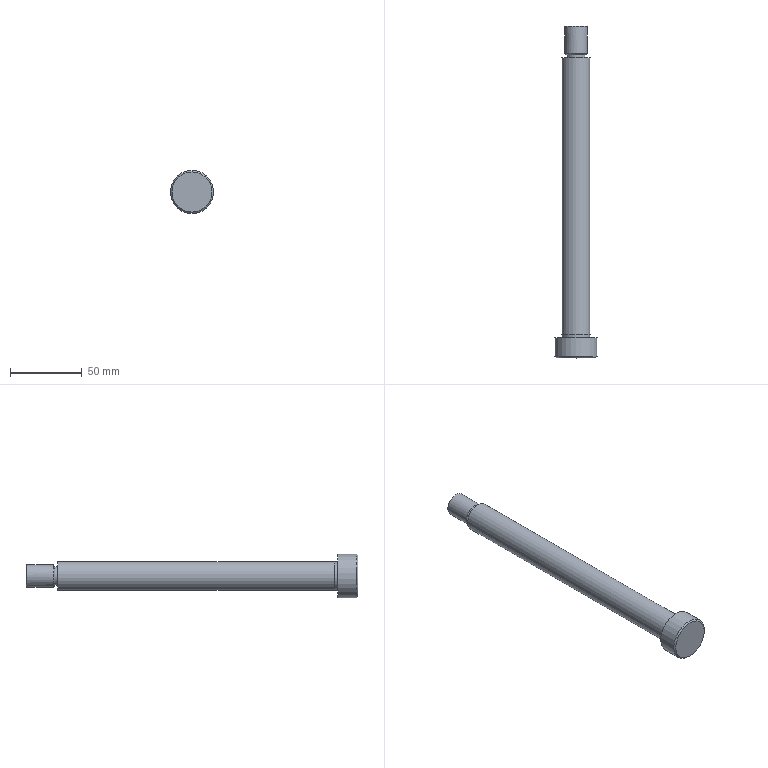Part | STEP file | SCREW-5_id334_x_t | 1 solid | 13 faces | box 30 x 231 x 30 mm | volume 75324 mm3 | plane 5 | cylinder 5 | cone 3 | commonest cylinder face diameters 13.2 x1 16 x1 19.5 x1 20 x1 30 x1
STEP:
#1=CARTESIAN_POINT('',(162.,-118.5,84.));
#2=VERTEX_POINT('',#1);
#3=CARTESIAN_POINT('',(162.,-118.5,70.));
#4=DIRECTION('',(0.,1.,0.));
#5=DIRECTION('',(0.,0.,1.));
#6=AXIS2_PLACEMENT_3D('',#3,#4,#5);
#7=CIRCLE('',#6,14.);
#8=EDGE_CURVE('',#2,#2,#7,.T.);
#9=ORIENTED_EDGE('',*,*,#8,.F.);
#10=EDGE_LOOP('',(#9));
#11=FACE_OUTER_BOUND('',#10,.T.);
#12=CARTESIAN_POINT('',(162.,-118.5,70.));
#13=DIRECTION('',(0.,-1.,0.));
#14=DIRECTION('',(0.,0.,-1.));
#15=AXIS2_PLACEMENT_3D('',#12,#13,#14);
#16=PLANE('',#15);
#17=ADVANCED_FACE('',(#11),#16,.T.);
#18=CARTESIAN_POINT('',(162.,112.5,63.));
#19=VERTEX_POINT('',#18);
#20=CARTESIAN_POINT('',(162.,112.5,70.));
#21=DIRECTION('',(0.,-1.,0.));
#22=DIRECTION('',(0.,0.,-1.));
#23=AXIS2_PLACEMENT_3D('',#20,#21,#22);
#24=CIRCLE('',#23,7.);
#25=EDGE_CURVE('',#19,#19,#24,.T.);
#26=ORIENTED_EDGE('',*,*,#25,.F.);
#27=EDGE_LOOP('',(#26));
#28=FACE_OUTER_BOUND('',#27,.T.);
#29=CARTESIAN_POINT('',(162.,112.5,70.));
#30=DIRECTION('',(0.,-1.,0.));
#31=DIRECTION('',(0.,0.,-1.));
#32=AXIS2_PLACEMENT_3D('',#29,#30,#31);
#33=PLANE('',#32);
#34=ADVANCED_FACE('',(#28),#33,.F.);
#35=ORIENTED_EDGE('',*,*,#8,.T.);
#36=EDGE_LOOP('',(#35));
#37=FACE_BOUND('',#36,.T.);
#38=CARTESIAN_POINT('',(162.,-117.5,55.));
#39=VERTEX_POINT('',#38);
#40=CARTESIAN_POINT('',(162.,-117.5,70.));
#41=DIRECTION('',(0.,1.,0.));
#42=DIRECTION('',(0.,0.,-1.));
#43=AXIS2_PLACEMENT_3D('',#40,#41,#42);
#44=CIRCLE('',#43,15.);
#45=EDGE_CURVE('',#39,#39,#44,.T.);
#46=ORIENTED_EDGE('',*,*,#45,.F.);
#47=EDGE_LOOP('',(#46));
#48=FACE_BOUND('',#47,.T.);
#49=CARTESIAN_POINT('',(162.,-117.5,70.));
#50=DIRECTION('',(0.,1.,0.));
#51=DIRECTION('',(0.,0.,1.));
#52=AXIS2_PLACEMENT_3D('',#49,#50,#51);
#53=CONICAL_SURFACE('',#52,15.,45.);
#54=ADVANCED_FACE('',(#37,#48),#53,.T.);
#55=ORIENTED_EDGE('',*,*,#25,.T.);
#56=EDGE_LOOP('',(#55));
#57=FACE_BOUND('',#56,.T.);
#58=CARTESIAN_POINT('',(162.,112.,62.));
#59=VERTEX_POINT('',#58);
#60=CARTESIAN_POINT('',(162.,112.,70.));
#61=DIRECTION('',(0.,-1.,0.));
#62=DIRECTION('',(0.,0.,-1.));
#63=AXIS2_PLACEMENT_3D('',#60,#61,#62);
#64=CIRCLE('',#63,8.);
#65=EDGE_CURVE('',#59,#59,#64,.T.);
#66=ORIENTED_EDGE('',*,*,#65,.F.);
#67=EDGE_LOOP('',(#66));
#68=FACE_BOUND('',#67,.T.);
#69=CARTESIAN_POINT('',(162.,112.,70.));
#70=DIRECTION('',(0.,-1.,0.));
#71=DIRECTION('',(0.,0.,-1.));
#72=AXIS2_PLACEMENT_3D('',#69,#70,#71);
#73=CONICAL_SURFACE('',#72,8.,63.435);
#74=ADVANCED_FACE('',(#57,#68),#73,.T.);
#75=ORIENTED_EDGE('',*,*,#45,.T.);
#76=EDGE_LOOP('',(#75));
#77=FACE_BOUND('',#76,.T.);
#78=CARTESIAN_POINT('',(162.,-104.5,55.));
#79=VERTEX_POINT('',#78);
#80=CARTESIAN_POINT('',(162.,-104.5,70.));
#81=DIRECTION('',(0.,-1.,0.));
#82=DIRECTION('',(0.,0.,-1.));
#83=AXIS2_PLACEMENT_3D('',#80,#81,#82);
#84=CIRCLE('',#83,15.);
#85=EDGE_CURVE('',#79,#79,#84,.T.);
#86=ORIENTED_EDGE('',*,*,#85,.T.);
#87=EDGE_LOOP('',(#86));
#88=FACE_BOUND('',#87,.T.);
#89=CARTESIAN_POINT('',(162.,-130.05,70.));
#90=DIRECTION('',(0.,-1.,0.));
#91=DIRECTION('',(0.,0.,-1.));
#92=AXIS2_PLACEMENT_3D('',#89,#90,#91);
#93=CYLINDRICAL_SURFACE('',#92,15.);
#94=ADVANCED_FACE('',(#77,#88),#93,.T.);
#95=ORIENTED_EDGE('',*,*,#65,.T.);
#96=EDGE_LOOP('',(#95));
#97=FACE_BOUND('',#96,.T.);
#98=CARTESIAN_POINT('',(170.,93.371,70.));
#99=VERTEX_POINT('',#98);
#100=CARTESIAN_POINT('',(162.,93.371,70.));
#101=DIRECTION('',(0.,-1.,0.));
#102=DIRECTION('',(1.,0.,0.));
#103=AXIS2_PLACEMENT_3D('',#100,#101,#102);
#104=CIRCLE('',#103,8.);
#105=EDGE_CURVE('',#99,#99,#104,.T.);
#106=ORIENTED_EDGE('',*,*,#105,.F.);
#107=EDGE_LOOP('',(#106));
#108=FACE_BOUND('',#107,.T.);
#109=CARTESIAN_POINT('',(162.,-130.05,70.));
#110=DIRECTION('',(0.,-1.,0.));
#111=DIRECTION('',(0.,0.,-1.));
#112=AXIS2_PLACEMENT_3D('',#109,#110,#111);
#113=CYLINDRICAL_SURFACE('',#112,8.);
#114=ADVANCED_FACE('',(#97,#108),#113,.T.);
#115=CARTESIAN_POINT('',(162.,-104.5,60.25));
#116=VERTEX_POINT('',#115);
#117=CARTESIAN_POINT('',(162.,-104.5,70.));
#118=DIRECTION('',(0.,1.,0.));
#119=DIRECTION('',(0.,0.,-1.));
#120=AXIS2_PLACEMENT_3D('',#117,#118,#119);
#121=CIRCLE('',#120,9.75);
#122=EDGE_CURVE('',#116,#116,#121,.T.);
#123=ORIENTED_EDGE('',*,*,#122,.F.);
#124=EDGE_LOOP('',(#123));
#125=FACE_BOUND('',#124,.T.);
#126=ORIENTED_EDGE('',*,*,#85,.F.);
#127=EDGE_LOOP('',(#126));
#128=FACE_BOUND('',#127,.T.);
#129=CARTESIAN_POINT('',(162.,-104.5,70.));
#130=DIRECTION('',(0.,-1.,0.));
#131=DIRECTION('',(0.,0.,-1.));
#132=AXIS2_PLACEMENT_3D('',#129,#130,#131);
#133=PLANE('',#132);
#134=ADVANCED_FACE('',(#125,#128),#133,.F.);
#135=ORIENTED_EDGE('',*,*,#105,.T.);
#136=EDGE_LOOP('',(#135));
#137=FACE_BOUND('',#136,.T.);
#138=CARTESIAN_POINT('',(162.,92.563,63.4));
#139=VERTEX_POINT('',#138);
#140=CARTESIAN_POINT('',(162.,92.563,70.));
#141=DIRECTION('',(0.,-1.,0.));
#142=DIRECTION('',(0.,0.,-1.));
#143=AXIS2_PLACEMENT_3D('',#140,#141,#142);
#144=CIRCLE('',#143,6.6);
#145=EDGE_CURVE('',#139,#139,#144,.T.);
#146=ORIENTED_EDGE('',*,*,#145,.F.);
#147=EDGE_LOOP('',(#146));
#148=FACE_BOUND('',#147,.T.);
#149=CARTESIAN_POINT('',(162.,93.371,70.));
#150=DIRECTION('',(0.,1.,0.));
#151=DIRECTION('',(0.,0.,1.));
#152=AXIS2_PLACEMENT_3D('',#149,#150,#151);
#153=CONICAL_SURFACE('',#152,8.,60.);
#154=ADVANCED_FACE('',(#137,#148),#153,.T.);
#155=CARTESIAN_POINT('',(162.,-102.,60.25));
#156=VERTEX_POINT('',#155);
#157=CARTESIAN_POINT('',(162.,-102.,70.));
#158=DIRECTION('',(0.,1.,0.));
#159=DIRECTION('',(0.,0.,-1.));
#160=AXIS2_PLACEMENT_3D('',#157,#158,#159);
#161=CIRCLE('',#160,9.75);
#162=EDGE_CURVE('',#156,#156,#161,.T.);
#163=ORIENTED_EDGE('',*,*,#162,.F.);
#164=EDGE_LOOP('',(#163));
#165=FACE_BOUND('',#164,.T.);
#166=ORIENTED_EDGE('',*,*,#122,.T.);
#167=EDGE_LOOP('',(#166));
#168=FACE_BOUND('',#167,.T.);
#169=CARTESIAN_POINT('',(162.,-130.05,70.));
#170=DIRECTION('',(0.,-1.,0.));
#171=DIRECTION('',(0.,0.,-1.));
#172=AXIS2_PLACEMENT_3D('',#169,#170,#171);
#173=CYLINDRICAL_SURFACE('',#172,9.75);
#174=ADVANCED_FACE('',(#165,#168),#173,.T.);
#175=ORIENTED_EDGE('',*,*,#145,.T.);
#176=EDGE_LOOP('',(#175));
#177=FACE_BOUND('',#176,.T.);
#178=CARTESIAN_POINT('',(162.,90.5,63.4));
#179=VERTEX_POINT('',#178);
#180=CARTESIAN_POINT('',(162.,90.5,70.));
#181=DIRECTION('',(0.,1.,0.));
#182=DIRECTION('',(0.,0.,-1.));
#183=AXIS2_PLACEMENT_3D('',#180,#181,#182);
#184=CIRCLE('',#183,6.6);
#185=EDGE_CURVE('',#179,#179,#184,.T.);
#186=ORIENTED_EDGE('',*,*,#185,.T.);
#187=EDGE_LOOP('',(#186));
#188=FACE_BOUND('',#187,.T.);
#189=CARTESIAN_POINT('',(162.,-130.05,70.));
#190=DIRECTION('',(0.,-1.,0.));
#191=DIRECTION('',(0.,0.,-1.));
#192=AXIS2_PLACEMENT_3D('',#189,#190,#191);
#193=CYLINDRICAL_SURFACE('',#192,6.6);
#194=ADVANCED_FACE('',(#177,#188),#193,.T.);
#195=ORIENTED_EDGE('',*,*,#162,.T.);
#196=EDGE_LOOP('',(#195));
#197=FACE_BOUND('',#196,.T.);
#198=CARTESIAN_POINT('',(162.,-102.,60.));
#199=VERTEX_POINT('',#198);
#200=CARTESIAN_POINT('',(162.,-102.,70.));
#201=DIRECTION('',(0.,1.,0.));
#202=DIRECTION('',(0.,0.,-1.));
#203=AXIS2_PLACEMENT_3D('',#200,#201,#202);
#204=CIRCLE('',#203,10.);
#205=EDGE_CURVE('',#199,#199,#204,.T.);
#206=ORIENTED_EDGE('',*,*,#205,.F.);
#207=EDGE_LOOP('',(#206));
#208=FACE_BOUND('',#207,.T.);
#209=CARTESIAN_POINT('',(162.,-102.,70.));
#210=DIRECTION('',(0.,-1.,0.));
#211=DIRECTION('',(0.,0.,-1.));
#212=AXIS2_PLACEMENT_3D('',#209,#210,#211);
#213=PLANE('',#212);
#214=ADVANCED_FACE('',(#197,#208),#213,.T.);
#215=ORIENTED_EDGE('',*,*,#185,.F.);
#216=EDGE_LOOP('',(#215));
#217=FACE_BOUND('',#216,.T.);
#218=CARTESIAN_POINT('',(162.,90.5,60.));
#219=VERTEX_POINT('',#218);
#220=CARTESIAN_POINT('',(162.,90.5,70.));
#221=DIRECTION('',(0.,-1.,0.));
#222=DIRECTION('',(0.,0.,-1.));
#223=AXIS2_PLACEMENT_3D('',#220,#221,#222);
#224=CIRCLE('',#223,10.);
#225=EDGE_CURVE('',#219,#219,#224,.T.);
#226=ORIENTED_EDGE('',*,*,#225,.F.);
#227=EDGE_LOOP('',(#226));
#228=FACE_BOUND('',#227,.T.);
#229=CARTESIAN_POINT('',(162.,90.5,70.));
#230=DIRECTION('',(0.,-1.,0.));
#231=DIRECTION('',(0.,0.,-1.));
#232=AXIS2_PLACEMENT_3D('',#229,#230,#231);
#233=PLANE('',#232);
#234=ADVANCED_FACE('',(#217,#228),#233,.F.);
#235=ORIENTED_EDGE('',*,*,#225,.T.);
#236=EDGE_LOOP('',(#235));
#237=FACE_BOUND('',#236,.T.);
#238=ORIENTED_EDGE('',*,*,#205,.T.);
#239=EDGE_LOOP('',(#238));
#240=FACE_BOUND('',#239,.T.);
#241=CARTESIAN_POINT('',(162.,-130.05,70.));
#242=DIRECTION('',(0.,-1.,0.));
#243=DIRECTION('',(0.,0.,-1.));
#244=AXIS2_PLACEMENT_3D('',#241,#242,#243);
#245=CYLINDRICAL_SURFACE('',#244,10.);
#246=ADVANCED_FACE('',(#237,#240),#245,.T.);
#247=CLOSED_SHELL('',(#17,#34,#54,#74,#94,#114,#134,#154,#174,#194,#214,#234,#246));
#248=MANIFOLD_SOLID_BREP('',#247);
#249=(LENGTH_UNIT()NAMED_UNIT(*)SI_UNIT(.MILLI.,.METRE.));
#250=UNCERTAINTY_MEASURE_WITH_UNIT(LENGTH_MEASURE(0.00002),#249,'','');
#251=(NAMED_UNIT(*)PLANE_ANGLE_UNIT()SI_UNIT($,.RADIAN.));
#252=PLANE_ANGLE_MEASURE_WITH_UNIT(PLANE_ANGLE_MEASURE(0.01745),#251);
#253=DIMENSIONAL_EXPONENTS(0.,0.,0.,0.,0.,0.,0.);
#254=(CONVERSION_BASED_UNIT('DEGREE',#252)NAMED_UNIT(#253)PLANE_ANGLE_UNIT());
#255=(NAMED_UNIT(*)SI_UNIT($,.STERADIAN.)SOLID_ANGLE_UNIT());
#256=(GEOMETRIC_REPRESENTATION_CONTEXT(3)GLOBAL_UNCERTAINTY_ASSIGNED_CONTEXT((#250))GLOBAL_UNIT_ASSIGNED_CONTEXT((#249,#254,#255))REPRESENTATION_CONTEXT('',''));
#257=ADVANCED_BREP_SHAPE_REPRESENTATION('',(#248),#256);